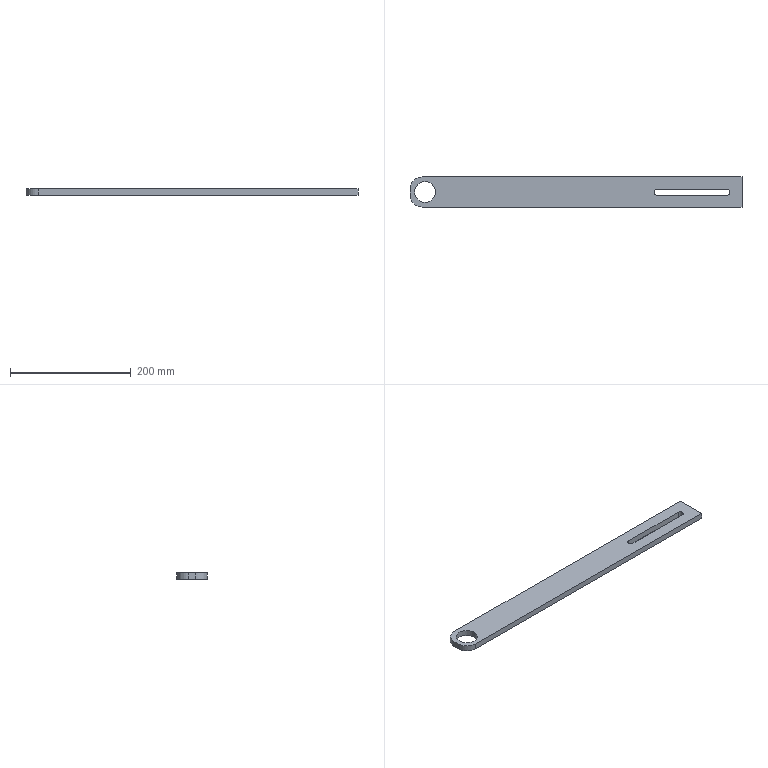Part | SolidWorks | features ICE 2, Extrusion 1, Fillet 1 | 1 solid | 18 faces | box 550 x 50 x 10 mm | volume 251336 mm3 | plane 10 | cylinder 8 | commonest cylinder face diameters 9 x4 35 x2 40 x2
STEP:
#1=CARTESIAN_POINT('',(-267.5,0.,0.));
#2=VERTEX_POINT('',#1);
#3=CARTESIAN_POINT('',(-232.5,0.,0.));
#4=VERTEX_POINT('',#3);
#5=CARTESIAN_POINT('',(-250.,0.,0.));
#6=DIRECTION('',(0.,0.,1.));
#7=DIRECTION('',(1.,0.,0.));
#8=AXIS2_PLACEMENT_3D('',#5,#6,#7);
#9=CIRCLE('',#8,17.5);
#10=EDGE_CURVE('',#2,#4,#9,.T.);
#11=ORIENTED_EDGE('',*,*,#10,.F.);
#12=CARTESIAN_POINT('',(-267.5,0.,10.));
#13=VERTEX_POINT('',#12);
#14=CARTESIAN_POINT('',(-267.5,0.,0.));
#15=DIRECTION('',(0.,0.,1.));
#16=VECTOR('',#15,1000.);
#17=LINE('',#14,#16);
#18=EDGE_CURVE('',#2,#13,#17,.T.);
#19=ORIENTED_EDGE('',*,*,#18,.T.);
#20=CARTESIAN_POINT('',(-232.5,0.,10.));
#21=VERTEX_POINT('',#20);
#22=CARTESIAN_POINT('',(-250.,0.,10.));
#23=DIRECTION('',(0.,0.,1.));
#24=DIRECTION('',(1.,0.,0.));
#25=AXIS2_PLACEMENT_3D('',#22,#23,#24);
#26=CIRCLE('',#25,17.5);
#27=EDGE_CURVE('',#13,#21,#26,.T.);
#28=ORIENTED_EDGE('',*,*,#27,.T.);
#29=CARTESIAN_POINT('',(-232.5,0.,0.));
#30=DIRECTION('',(0.,0.,1.));
#31=VECTOR('',#30,1000.);
#32=LINE('',#29,#31);
#33=EDGE_CURVE('',#4,#21,#32,.T.);
#34=ORIENTED_EDGE('',*,*,#33,.F.);
#35=EDGE_LOOP('',(#11,#19,#28,#34));
#36=FACE_OUTER_BOUND('',#35,.T.);
#37=CARTESIAN_POINT('',(-250.,0.,0.));
#38=DIRECTION('',(0.,0.,1.));
#39=DIRECTION('',(1.,0.,0.));
#40=AXIS2_PLACEMENT_3D('',#37,#38,#39);
#41=CYLINDRICAL_SURFACE('',#40,17.5);
#42=ADVANCED_FACE('',(#36),#41,.F.);
#43=CARTESIAN_POINT('',(-275.,5.,0.));
#44=VERTEX_POINT('',#43);
#45=CARTESIAN_POINT('',(-275.,-5.,0.));
#46=VERTEX_POINT('',#45);
#47=CARTESIAN_POINT('',(-275.,-25.,0.));
#48=DIRECTION('',(0.,-1.,0.));
#49=VECTOR('',#48,1000.);
#50=LINE('',#47,#49);
#51=EDGE_CURVE('',#44,#46,#50,.T.);
#52=ORIENTED_EDGE('',*,*,#51,.T.);
#53=CARTESIAN_POINT('',(-275.,-5.,10.));
#54=VERTEX_POINT('',#53);
#55=CARTESIAN_POINT('',(-275.,-5.,10.));
#56=DIRECTION('',(0.,0.,1.));
#57=VECTOR('',#56,1000.);
#58=LINE('',#55,#57);
#59=EDGE_CURVE('',#46,#54,#58,.T.);
#60=ORIENTED_EDGE('',*,*,#59,.T.);
#61=CARTESIAN_POINT('',(-275.,5.,10.));
#62=VERTEX_POINT('',#61);
#63=CARTESIAN_POINT('',(-275.,-25.,10.));
#64=DIRECTION('',(0.,-1.,0.));
#65=VECTOR('',#64,1000.);
#66=LINE('',#63,#65);
#67=EDGE_CURVE('',#62,#54,#66,.T.);
#68=ORIENTED_EDGE('',*,*,#67,.F.);
#69=CARTESIAN_POINT('',(-275.,5.,10.));
#70=DIRECTION('',(0.,0.,-1.));
#71=VECTOR('',#70,1000.);
#72=LINE('',#69,#71);
#73=EDGE_CURVE('',#62,#44,#72,.T.);
#74=ORIENTED_EDGE('',*,*,#73,.T.);
#75=EDGE_LOOP('',(#52,#60,#68,#74));
#76=FACE_OUTER_BOUND('',#75,.T.);
#77=CARTESIAN_POINT('',(-275.,-25.,10.));
#78=DIRECTION('',(1.,0.,0.));
#79=DIRECTION('',(0.,0.,-1.));
#80=AXIS2_PLACEMENT_3D('',#77,#78,#79);
#81=PLANE('',#80);
#82=ADVANCED_FACE('',(#76),#81,.F.);
#83=CARTESIAN_POINT('',(-255.,-25.,10.));
#84=VERTEX_POINT('',#83);
#85=CARTESIAN_POINT('',(275.,-25.,10.));
#86=VERTEX_POINT('',#85);
#87=CARTESIAN_POINT('',(275.,-25.,10.));
#88=DIRECTION('',(1.,0.,0.));
#89=VECTOR('',#88,1000.);
#90=LINE('',#87,#89);
#91=EDGE_CURVE('',#84,#86,#90,.T.);
#92=ORIENTED_EDGE('',*,*,#91,.F.);
#93=CARTESIAN_POINT('',(-255.,-25.,0.));
#94=VERTEX_POINT('',#93);
#95=CARTESIAN_POINT('',(-255.,-25.,10.));
#96=DIRECTION('',(0.,0.,-1.));
#97=VECTOR('',#96,1000.);
#98=LINE('',#95,#97);
#99=EDGE_CURVE('',#84,#94,#98,.T.);
#100=ORIENTED_EDGE('',*,*,#99,.T.);
#101=CARTESIAN_POINT('',(275.,-25.,0.));
#102=VERTEX_POINT('',#101);
#103=CARTESIAN_POINT('',(275.,-25.,0.));
#104=DIRECTION('',(1.,0.,0.));
#105=VECTOR('',#104,1000.);
#106=LINE('',#103,#105);
#107=EDGE_CURVE('',#94,#102,#106,.T.);
#108=ORIENTED_EDGE('',*,*,#107,.T.);
#109=CARTESIAN_POINT('',(275.,-25.,10.));
#110=DIRECTION('',(0.,0.,-1.));
#111=VECTOR('',#110,1000.);
#112=LINE('',#109,#111);
#113=EDGE_CURVE('',#86,#102,#112,.T.);
#114=ORIENTED_EDGE('',*,*,#113,.F.);
#115=EDGE_LOOP('',(#92,#100,#108,#114));
#116=FACE_OUTER_BOUND('',#115,.T.);
#117=CARTESIAN_POINT('',(275.,-25.,10.));
#118=DIRECTION('',(0.,1.,0.));
#119=DIRECTION('',(-1.,0.,0.));
#120=AXIS2_PLACEMENT_3D('',#117,#118,#119);
#121=PLANE('',#120);
#122=ADVANCED_FACE('',(#116),#121,.F.);
#123=CARTESIAN_POINT('',(275.,25.,0.));
#124=VERTEX_POINT('',#123);
#125=CARTESIAN_POINT('',(275.,-25.,0.));
#126=DIRECTION('',(0.,1.,0.));
#127=VECTOR('',#126,1000.);
#128=LINE('',#125,#127);
#129=EDGE_CURVE('',#102,#124,#128,.T.);
#130=ORIENTED_EDGE('',*,*,#129,.T.);
#131=CARTESIAN_POINT('',(275.,25.,10.));
#132=VERTEX_POINT('',#131);
#133=CARTESIAN_POINT('',(275.,25.,10.));
#134=DIRECTION('',(0.,0.,-1.));
#135=VECTOR('',#134,1000.);
#136=LINE('',#133,#135);
#137=EDGE_CURVE('',#132,#124,#136,.T.);
#138=ORIENTED_EDGE('',*,*,#137,.F.);
#139=CARTESIAN_POINT('',(275.,-25.,10.));
#140=DIRECTION('',(0.,1.,0.));
#141=VECTOR('',#140,1000.);
#142=LINE('',#139,#141);
#143=EDGE_CURVE('',#86,#132,#142,.T.);
#144=ORIENTED_EDGE('',*,*,#143,.F.);
#145=ORIENTED_EDGE('',*,*,#113,.T.);
#146=EDGE_LOOP('',(#130,#138,#144,#145));
#147=FACE_OUTER_BOUND('',#146,.T.);
#148=CARTESIAN_POINT('',(275.,-25.,10.));
#149=DIRECTION('',(-1.,0.,0.));
#150=DIRECTION('',(0.,0.,1.));
#151=AXIS2_PLACEMENT_3D('',#148,#149,#150);
#152=PLANE('',#151);
#153=ADVANCED_FACE('',(#147),#152,.F.);
#154=CARTESIAN_POINT('',(-255.,25.,0.));
#155=VERTEX_POINT('',#154);
#156=CARTESIAN_POINT('',(275.,25.,0.));
#157=DIRECTION('',(-1.,0.,0.));
#158=VECTOR('',#157,1000.);
#159=LINE('',#156,#158);
#160=EDGE_CURVE('',#124,#155,#159,.T.);
#161=ORIENTED_EDGE('',*,*,#160,.T.);
#162=CARTESIAN_POINT('',(-255.,25.,10.));
#163=VERTEX_POINT('',#162);
#164=CARTESIAN_POINT('',(-255.,25.,10.));
#165=DIRECTION('',(0.,0.,1.));
#166=VECTOR('',#165,1000.);
#167=LINE('',#164,#166);
#168=EDGE_CURVE('',#155,#163,#167,.T.);
#169=ORIENTED_EDGE('',*,*,#168,.T.);
#170=CARTESIAN_POINT('',(275.,25.,10.));
#171=DIRECTION('',(-1.,0.,0.));
#172=VECTOR('',#171,1000.);
#173=LINE('',#170,#172);
#174=EDGE_CURVE('',#132,#163,#173,.T.);
#175=ORIENTED_EDGE('',*,*,#174,.F.);
#176=ORIENTED_EDGE('',*,*,#137,.T.);
#177=EDGE_LOOP('',(#161,#169,#175,#176));
#178=FACE_OUTER_BOUND('',#177,.T.);
#179=CARTESIAN_POINT('',(275.,25.,10.));
#180=DIRECTION('',(0.,-1.,0.));
#181=DIRECTION('',(1.,0.,0.));
#182=AXIS2_PLACEMENT_3D('',#179,#180,#181);
#183=PLANE('',#182);
#184=ADVANCED_FACE('',(#178),#183,.F.);
#185=CARTESIAN_POINT('',(250.1,-5.341,10.));
#186=VERTEX_POINT('',#185);
#187=CARTESIAN_POINT('',(254.6,-0.841,10.));
#188=VERTEX_POINT('',#187);
#189=CARTESIAN_POINT('',(250.1,-0.841,10.));
#190=DIRECTION('',(0.,0.,1.));
#191=DIRECTION('',(1.,0.,0.));
#192=AXIS2_PLACEMENT_3D('',#189,#190,#191);
#193=CIRCLE('',#192,4.5);
#194=EDGE_CURVE('',#186,#188,#193,.T.);
#195=ORIENTED_EDGE('',*,*,#194,.F.);
#196=CARTESIAN_POINT('',(134.1,-5.341,10.));
#197=VERTEX_POINT('',#196);
#198=CARTESIAN_POINT('',(250.1,-5.341,10.));
#199=DIRECTION('',(1.,0.,0.));
#200=VECTOR('',#199,1000.);
#201=LINE('',#198,#200);
#202=EDGE_CURVE('',#197,#186,#201,.T.);
#203=ORIENTED_EDGE('',*,*,#202,.F.);
#204=CARTESIAN_POINT('',(129.6,-0.841,10.));
#205=VERTEX_POINT('',#204);
#206=CARTESIAN_POINT('',(134.1,-0.841,10.));
#207=DIRECTION('',(0.,0.,1.));
#208=DIRECTION('',(-1.,0.,0.));
#209=AXIS2_PLACEMENT_3D('',#206,#207,#208);
#210=CIRCLE('',#209,4.5);
#211=EDGE_CURVE('',#205,#197,#210,.T.);
#212=ORIENTED_EDGE('',*,*,#211,.F.);
#213=CARTESIAN_POINT('',(129.6,0.159,10.));
#214=VERTEX_POINT('',#213);
#215=CARTESIAN_POINT('',(129.6,-0.841,10.));
#216=DIRECTION('',(0.,-1.,0.));
#217=VECTOR('',#216,1000.);
#218=LINE('',#215,#217);
#219=EDGE_CURVE('',#214,#205,#218,.T.);
#220=ORIENTED_EDGE('',*,*,#219,.F.);
#221=CARTESIAN_POINT('',(134.1,4.659,10.));
#222=VERTEX_POINT('',#221);
#223=CARTESIAN_POINT('',(134.1,0.159,10.));
#224=DIRECTION('',(0.,0.,1.));
#225=DIRECTION('',(1.,0.,0.));
#226=AXIS2_PLACEMENT_3D('',#223,#224,#225);
#227=CIRCLE('',#226,4.5);
#228=EDGE_CURVE('',#222,#214,#227,.T.);
#229=ORIENTED_EDGE('',*,*,#228,.F.);
#230=CARTESIAN_POINT('',(250.1,4.659,10.));
#231=VERTEX_POINT('',#230);
#232=CARTESIAN_POINT('',(250.1,4.659,10.));
#233=DIRECTION('',(-1.,0.,0.));
#234=VECTOR('',#233,1000.);
#235=LINE('',#232,#234);
#236=EDGE_CURVE('',#231,#222,#235,.T.);
#237=ORIENTED_EDGE('',*,*,#236,.F.);
#238=CARTESIAN_POINT('',(254.6,0.159,10.));
#239=VERTEX_POINT('',#238);
#240=CARTESIAN_POINT('',(250.1,0.159,10.));
#241=DIRECTION('',(0.,0.,1.));
#242=DIRECTION('',(1.,0.,0.));
#243=AXIS2_PLACEMENT_3D('',#240,#241,#242);
#244=CIRCLE('',#243,4.5);
#245=EDGE_CURVE('',#239,#231,#244,.T.);
#246=ORIENTED_EDGE('',*,*,#245,.F.);
#247=CARTESIAN_POINT('',(254.6,-0.841,10.));
#248=DIRECTION('',(0.,1.,0.));
#249=VECTOR('',#248,1000.);
#250=LINE('',#247,#249);
#251=EDGE_CURVE('',#188,#239,#250,.T.);
#252=ORIENTED_EDGE('',*,*,#251,.F.);
#253=EDGE_LOOP('',(#195,#203,#212,#220,#229,#237,#246,#252));
#254=FACE_BOUND('',#253,.T.);
#255=CARTESIAN_POINT('',(-250.,0.,10.));
#256=DIRECTION('',(0.,0.,1.));
#257=DIRECTION('',(1.,0.,0.));
#258=AXIS2_PLACEMENT_3D('',#255,#256,#257);
#259=CIRCLE('',#258,17.5);
#260=EDGE_CURVE('',#21,#13,#259,.T.);
#261=ORIENTED_EDGE('',*,*,#260,.F.);
#262=ORIENTED_EDGE('',*,*,#27,.F.);
#263=EDGE_LOOP('',(#261,#262));
#264=FACE_BOUND('',#263,.T.);
#265=ORIENTED_EDGE('',*,*,#67,.T.);
#266=CARTESIAN_POINT('',(-255.,-5.,10.));
#267=DIRECTION('',(0.,0.,1.));
#268=DIRECTION('',(1.,0.,0.));
#269=AXIS2_PLACEMENT_3D('',#266,#267,#268);
#270=CIRCLE('',#269,20.);
#271=EDGE_CURVE('',#54,#84,#270,.T.);
#272=ORIENTED_EDGE('',*,*,#271,.T.);
#273=ORIENTED_EDGE('',*,*,#91,.T.);
#274=ORIENTED_EDGE('',*,*,#143,.T.);
#275=ORIENTED_EDGE('',*,*,#174,.T.);
#276=CARTESIAN_POINT('',(-255.,5.,10.));
#277=DIRECTION('',(0.,0.,1.));
#278=DIRECTION('',(1.,0.,0.));
#279=AXIS2_PLACEMENT_3D('',#276,#277,#278);
#280=CIRCLE('',#279,20.);
#281=EDGE_CURVE('',#163,#62,#280,.T.);
#282=ORIENTED_EDGE('',*,*,#281,.T.);
#283=EDGE_LOOP('',(#265,#272,#273,#274,#275,#282));
#284=FACE_OUTER_BOUND('',#283,.T.);
#285=CARTESIAN_POINT('',(-275.,25.,10.));
#286=DIRECTION('',(0.,0.,1.));
#287=DIRECTION('',(1.,0.,0.));
#288=AXIS2_PLACEMENT_3D('',#285,#286,#287);
#289=PLANE('',#288);
#290=ADVANCED_FACE('',(#254,#264,#284),#289,.T.);
#291=CARTESIAN_POINT('',(134.1,-5.341,0.));
#292=VERTEX_POINT('',#291);
#293=CARTESIAN_POINT('',(250.1,-5.341,0.));
#294=VERTEX_POINT('',#293);
#295=CARTESIAN_POINT('',(250.1,-5.341,0.));
#296=DIRECTION('',(1.,0.,0.));
#297=VECTOR('',#296,1000.);
#298=LINE('',#295,#297);
#299=EDGE_CURVE('',#292,#294,#298,.T.);
#300=ORIENTED_EDGE('',*,*,#299,.T.);
#301=CARTESIAN_POINT('',(254.6,-0.841,0.));
#302=VERTEX_POINT('',#301);
#303=CARTESIAN_POINT('',(250.1,-0.841,0.));
#304=DIRECTION('',(0.,0.,1.));
#305=DIRECTION('',(1.,0.,0.));
#306=AXIS2_PLACEMENT_3D('',#303,#304,#305);
#307=CIRCLE('',#306,4.5);
#308=EDGE_CURVE('',#294,#302,#307,.T.);
#309=ORIENTED_EDGE('',*,*,#308,.T.);
#310=CARTESIAN_POINT('',(254.6,0.159,0.));
#311=VERTEX_POINT('',#310);
#312=CARTESIAN_POINT('',(254.6,-0.841,0.));
#313=DIRECTION('',(0.,1.,0.));
#314=VECTOR('',#313,1000.);
#315=LINE('',#312,#314);
#316=EDGE_CURVE('',#302,#311,#315,.T.);
#317=ORIENTED_EDGE('',*,*,#316,.T.);
#318=CARTESIAN_POINT('',(250.1,4.659,0.));
#319=VERTEX_POINT('',#318);
#320=CARTESIAN_POINT('',(250.1,0.159,0.));
#321=DIRECTION('',(0.,0.,1.));
#322=DIRECTION('',(1.,0.,0.));
#323=AXIS2_PLACEMENT_3D('',#320,#321,#322);
#324=CIRCLE('',#323,4.5);
#325=EDGE_CURVE('',#311,#319,#324,.T.);
#326=ORIENTED_EDGE('',*,*,#325,.T.);
#327=CARTESIAN_POINT('',(134.1,4.659,0.));
#328=VERTEX_POINT('',#327);
#329=CARTESIAN_POINT('',(250.1,4.659,0.));
#330=DIRECTION('',(-1.,0.,0.));
#331=VECTOR('',#330,1000.);
#332=LINE('',#329,#331);
#333=EDGE_CURVE('',#319,#328,#332,.T.);
#334=ORIENTED_EDGE('',*,*,#333,.T.);
#335=CARTESIAN_POINT('',(129.6,0.159,0.));
#336=VERTEX_POINT('',#335);
#337=CARTESIAN_POINT('',(134.1,0.159,0.));
#338=DIRECTION('',(0.,0.,1.));
#339=DIRECTION('',(1.,0.,0.));
#340=AXIS2_PLACEMENT_3D('',#337,#338,#339);
#341=CIRCLE('',#340,4.5);
#342=EDGE_CURVE('',#328,#336,#341,.T.);
#343=ORIENTED_EDGE('',*,*,#342,.T.);
#344=CARTESIAN_POINT('',(129.6,-0.841,0.));
#345=VERTEX_POINT('',#344);
#346=CARTESIAN_POINT('',(129.6,-0.841,0.));
#347=DIRECTION('',(0.,-1.,0.));
#348=VECTOR('',#347,1000.);
#349=LINE('',#346,#348);
#350=EDGE_CURVE('',#336,#345,#349,.T.);
#351=ORIENTED_EDGE('',*,*,#350,.T.);
#352=CARTESIAN_POINT('',(134.1,-0.841,0.));
#353=DIRECTION('',(0.,0.,1.));
#354=DIRECTION('',(-1.,0.,0.));
#355=AXIS2_PLACEMENT_3D('',#352,#353,#354);
#356=CIRCLE('',#355,4.5);
#357=EDGE_CURVE('',#345,#292,#356,.T.);
#358=ORIENTED_EDGE('',*,*,#357,.T.);
#359=EDGE_LOOP('',(#300,#309,#317,#326,#334,#343,#351,#358));
#360=FACE_BOUND('',#359,.T.);
#361=CARTESIAN_POINT('',(-250.,0.,0.));
#362=DIRECTION('',(0.,0.,1.));
#363=DIRECTION('',(1.,0.,0.));
#364=AXIS2_PLACEMENT_3D('',#361,#362,#363);
#365=CIRCLE('',#364,17.5);
#366=EDGE_CURVE('',#4,#2,#365,.T.);
#367=ORIENTED_EDGE('',*,*,#366,.T.);
#368=ORIENTED_EDGE('',*,*,#10,.T.);
#369=EDGE_LOOP('',(#367,#368));
#370=FACE_BOUND('',#369,.T.);
#371=ORIENTED_EDGE('',*,*,#107,.F.);
#372=CARTESIAN_POINT('',(-255.,-5.,0.));
#373=DIRECTION('',(0.,0.,-1.));
#374=DIRECTION('',(1.,0.,0.));
#375=AXIS2_PLACEMENT_3D('',#372,#373,#374);
#376=CIRCLE('',#375,20.);
#377=EDGE_CURVE('',#94,#46,#376,.T.);
#378=ORIENTED_EDGE('',*,*,#377,.T.);
#379=ORIENTED_EDGE('',*,*,#51,.F.);
#380=CARTESIAN_POINT('',(-255.,5.,0.));
#381=DIRECTION('',(0.,0.,-1.));
#382=DIRECTION('',(1.,0.,0.));
#383=AXIS2_PLACEMENT_3D('',#380,#381,#382);
#384=CIRCLE('',#383,20.);
#385=EDGE_CURVE('',#44,#155,#384,.T.);
#386=ORIENTED_EDGE('',*,*,#385,.T.);
#387=ORIENTED_EDGE('',*,*,#160,.F.);
#388=ORIENTED_EDGE('',*,*,#129,.F.);
#389=EDGE_LOOP('',(#371,#378,#379,#386,#387,#388));
#390=FACE_OUTER_BOUND('',#389,.T.);
#391=CARTESIAN_POINT('',(-275.,25.,0.));
#392=DIRECTION('',(0.,0.,1.));
#393=DIRECTION('',(1.,0.,0.));
#394=AXIS2_PLACEMENT_3D('',#391,#392,#393);
#395=PLANE('',#394);
#396=ADVANCED_FACE('',(#360,#370,#390),#395,.F.);
#397=ORIENTED_EDGE('',*,*,#18,.F.);
#398=ORIENTED_EDGE('',*,*,#366,.F.);
#399=ORIENTED_EDGE('',*,*,#33,.T.);
#400=ORIENTED_EDGE('',*,*,#260,.T.);
#401=EDGE_LOOP('',(#397,#398,#399,#400));
#402=FACE_OUTER_BOUND('',#401,.T.);
#403=CARTESIAN_POINT('',(-250.,0.,0.));
#404=DIRECTION('',(0.,0.,1.));
#405=DIRECTION('',(1.,0.,0.));
#406=AXIS2_PLACEMENT_3D('',#403,#404,#405);
#407=CYLINDRICAL_SURFACE('',#406,17.5);
#408=ADVANCED_FACE('',(#402),#407,.F.);
#409=ORIENTED_EDGE('',*,*,#194,.T.);
#410=CARTESIAN_POINT('',(254.6,-0.841,0.));
#411=DIRECTION('',(0.,0.,1.));
#412=VECTOR('',#411,1000.);
#413=LINE('',#410,#412);
#414=EDGE_CURVE('',#302,#188,#413,.T.);
#415=ORIENTED_EDGE('',*,*,#414,.F.);
#416=ORIENTED_EDGE('',*,*,#308,.F.);
#417=CARTESIAN_POINT('',(250.1,-5.341,0.));
#418=DIRECTION('',(0.,0.,1.));
#419=VECTOR('',#418,1000.);
#420=LINE('',#417,#419);
#421=EDGE_CURVE('',#294,#186,#420,.T.);
#422=ORIENTED_EDGE('',*,*,#421,.T.);
#423=EDGE_LOOP('',(#409,#415,#416,#422));
#424=FACE_OUTER_BOUND('',#423,.T.);
#425=CARTESIAN_POINT('',(250.1,-0.841,0.));
#426=DIRECTION('',(0.,0.,1.));
#427=DIRECTION('',(1.,0.,0.));
#428=AXIS2_PLACEMENT_3D('',#425,#426,#427);
#429=CYLINDRICAL_SURFACE('',#428,4.5);
#430=ADVANCED_FACE('',(#424),#429,.F.);
#431=ORIENTED_EDGE('',*,*,#202,.T.);
#432=ORIENTED_EDGE('',*,*,#421,.F.);
#433=ORIENTED_EDGE('',*,*,#299,.F.);
#434=CARTESIAN_POINT('',(134.1,-5.341,0.));
#435=DIRECTION('',(0.,0.,1.));
#436=VECTOR('',#435,1000.);
#437=LINE('',#434,#436);
#438=EDGE_CURVE('',#292,#197,#437,.T.);
#439=ORIENTED_EDGE('',*,*,#438,.T.);
#440=EDGE_LOOP('',(#431,#432,#433,#439));
#441=FACE_OUTER_BOUND('',#440,.T.);
#442=CARTESIAN_POINT('',(250.1,-5.341,0.));
#443=DIRECTION('',(0.,-1.,0.));
#444=DIRECTION('',(1.,0.,0.));
#445=AXIS2_PLACEMENT_3D('',#442,#443,#444);
#446=PLANE('',#445);
#447=ADVANCED_FACE('',(#441),#446,.F.);
#448=ORIENTED_EDGE('',*,*,#211,.T.);
#449=ORIENTED_EDGE('',*,*,#438,.F.);
#450=ORIENTED_EDGE('',*,*,#357,.F.);
#451=CARTESIAN_POINT('',(129.6,-0.841,0.));
#452=DIRECTION('',(0.,0.,1.));
#453=VECTOR('',#452,1000.);
#454=LINE('',#451,#453);
#455=EDGE_CURVE('',#345,#205,#454,.T.);
#456=ORIENTED_EDGE('',*,*,#455,.T.);
#457=EDGE_LOOP('',(#448,#449,#450,#456));
#458=FACE_OUTER_BOUND('',#457,.T.);
#459=CARTESIAN_POINT('',(134.1,-0.841,0.));
#460=DIRECTION('',(0.,0.,1.));
#461=DIRECTION('',(1.,0.,0.));
#462=AXIS2_PLACEMENT_3D('',#459,#460,#461);
#463=CYLINDRICAL_SURFACE('',#462,4.5);
#464=ADVANCED_FACE('',(#458),#463,.F.);
#465=ORIENTED_EDGE('',*,*,#219,.T.);
#466=ORIENTED_EDGE('',*,*,#455,.F.);
#467=ORIENTED_EDGE('',*,*,#350,.F.);
#468=CARTESIAN_POINT('',(129.6,0.159,0.));
#469=DIRECTION('',(0.,0.,1.));
#470=VECTOR('',#469,1000.);
#471=LINE('',#468,#470);
#472=EDGE_CURVE('',#336,#214,#471,.T.);
#473=ORIENTED_EDGE('',*,*,#472,.T.);
#474=EDGE_LOOP('',(#465,#466,#467,#473));
#475=FACE_OUTER_BOUND('',#474,.T.);
#476=CARTESIAN_POINT('',(129.6,-0.841,0.));
#477=DIRECTION('',(-1.,0.,0.));
#478=DIRECTION('',(0.,0.,1.));
#479=AXIS2_PLACEMENT_3D('',#476,#477,#478);
#480=PLANE('',#479);
#481=ADVANCED_FACE('',(#475),#480,.F.);
#482=ORIENTED_EDGE('',*,*,#228,.T.);
#483=ORIENTED_EDGE('',*,*,#472,.F.);
#484=ORIENTED_EDGE('',*,*,#342,.F.);
#485=CARTESIAN_POINT('',(134.1,4.659,0.));
#486=DIRECTION('',(0.,0.,1.));
#487=VECTOR('',#486,1000.);
#488=LINE('',#485,#487);
#489=EDGE_CURVE('',#328,#222,#488,.T.);
#490=ORIENTED_EDGE('',*,*,#489,.T.);
#491=EDGE_LOOP('',(#482,#483,#484,#490));
#492=FACE_OUTER_BOUND('',#491,.T.);
#493=CARTESIAN_POINT('',(134.1,0.159,0.));
#494=DIRECTION('',(0.,0.,1.));
#495=DIRECTION('',(1.,0.,0.));
#496=AXIS2_PLACEMENT_3D('',#493,#494,#495);
#497=CYLINDRICAL_SURFACE('',#496,4.5);
#498=ADVANCED_FACE('',(#492),#497,.F.);
#499=ORIENTED_EDGE('',*,*,#236,.T.);
#500=ORIENTED_EDGE('',*,*,#489,.F.);
#501=ORIENTED_EDGE('',*,*,#333,.F.);
#502=CARTESIAN_POINT('',(250.1,4.659,0.));
#503=DIRECTION('',(0.,0.,1.));
#504=VECTOR('',#503,1000.);
#505=LINE('',#502,#504);
#506=EDGE_CURVE('',#319,#231,#505,.T.);
#507=ORIENTED_EDGE('',*,*,#506,.T.);
#508=EDGE_LOOP('',(#499,#500,#501,#507));
#509=FACE_OUTER_BOUND('',#508,.T.);
#510=CARTESIAN_POINT('',(250.1,4.659,0.));
#511=DIRECTION('',(0.,1.,0.));
#512=DIRECTION('',(-1.,0.,0.));
#513=AXIS2_PLACEMENT_3D('',#510,#511,#512);
#514=PLANE('',#513);
#515=ADVANCED_FACE('',(#509),#514,.F.);
#516=ORIENTED_EDGE('',*,*,#245,.T.);
#517=ORIENTED_EDGE('',*,*,#506,.F.);
#518=ORIENTED_EDGE('',*,*,#325,.F.);
#519=CARTESIAN_POINT('',(254.6,0.159,0.));
#520=DIRECTION('',(0.,0.,1.));
#521=VECTOR('',#520,1000.);
#522=LINE('',#519,#521);
#523=EDGE_CURVE('',#311,#239,#522,.T.);
#524=ORIENTED_EDGE('',*,*,#523,.T.);
#525=EDGE_LOOP('',(#516,#517,#518,#524));
#526=FACE_OUTER_BOUND('',#525,.T.);
#527=CARTESIAN_POINT('',(250.1,0.159,0.));
#528=DIRECTION('',(0.,0.,1.));
#529=DIRECTION('',(1.,0.,0.));
#530=AXIS2_PLACEMENT_3D('',#527,#528,#529);
#531=CYLINDRICAL_SURFACE('',#530,4.5);
#532=ADVANCED_FACE('',(#526),#531,.F.);
#533=ORIENTED_EDGE('',*,*,#251,.T.);
#534=ORIENTED_EDGE('',*,*,#523,.F.);
#535=ORIENTED_EDGE('',*,*,#316,.F.);
#536=ORIENTED_EDGE('',*,*,#414,.T.);
#537=EDGE_LOOP('',(#533,#534,#535,#536));
#538=FACE_OUTER_BOUND('',#537,.T.);
#539=CARTESIAN_POINT('',(254.6,-0.841,0.));
#540=DIRECTION('',(1.,0.,0.));
#541=DIRECTION('',(0.,0.,-1.));
#542=AXIS2_PLACEMENT_3D('',#539,#540,#541);
#543=PLANE('',#542);
#544=ADVANCED_FACE('',(#538),#543,.F.);
#545=ORIENTED_EDGE('',*,*,#271,.F.);
#546=ORIENTED_EDGE('',*,*,#59,.F.);
#547=ORIENTED_EDGE('',*,*,#377,.F.);
#548=ORIENTED_EDGE('',*,*,#99,.F.);
#549=EDGE_LOOP('',(#545,#546,#547,#548));
#550=FACE_OUTER_BOUND('',#549,.T.);
#551=CARTESIAN_POINT('',(-255.,-5.,10.));
#552=DIRECTION('',(0.,0.,-1.));
#553=DIRECTION('',(-1.,0.,0.));
#554=AXIS2_PLACEMENT_3D('',#551,#552,#553);
#555=CYLINDRICAL_SURFACE('',#554,20.);
#556=ADVANCED_FACE('',(#550),#555,.T.);
#557=ORIENTED_EDGE('',*,*,#281,.F.);
#558=ORIENTED_EDGE('',*,*,#168,.F.);
#559=ORIENTED_EDGE('',*,*,#385,.F.);
#560=ORIENTED_EDGE('',*,*,#73,.F.);
#561=EDGE_LOOP('',(#557,#558,#559,#560));
#562=FACE_OUTER_BOUND('',#561,.T.);
#563=CARTESIAN_POINT('',(-255.,5.,10.));
#564=DIRECTION('',(0.,0.,-1.));
#565=DIRECTION('',(-1.,0.,0.));
#566=AXIS2_PLACEMENT_3D('',#563,#564,#565);
#567=CYLINDRICAL_SURFACE('',#566,20.);
#568=ADVANCED_FACE('',(#562),#567,.T.);
#569=CLOSED_SHELL('',(#42,#82,#122,#153,#184,#290,#396,#408,#430,#447,#464,#481,#498,#515,#532,#544,#556,#568));
#570=MANIFOLD_SOLID_BREP('',#569);
#571=CARTESIAN_POINT('',(0.,0.,0.));
#572=DIRECTION('',(0.,0.,1.));
#573=DIRECTION('',(1.,0.,0.));
#574=AXIS2_PLACEMENT_3D('',#571,#572,#573);
#575=(LENGTH_UNIT()NAMED_UNIT(*)SI_UNIT(.MILLI.,.METRE.));
#576=UNCERTAINTY_MEASURE_WITH_UNIT(LENGTH_MEASURE(0.00001),#575,'','');
#577=(NAMED_UNIT(*)PLANE_ANGLE_UNIT()SI_UNIT($,.RADIAN.));
#578=(NAMED_UNIT(*)SI_UNIT($,.STERADIAN.)SOLID_ANGLE_UNIT());
#579=(GEOMETRIC_REPRESENTATION_CONTEXT(3)GLOBAL_UNCERTAINTY_ASSIGNED_CONTEXT((#576))GLOBAL_UNIT_ASSIGNED_CONTEXT((#575,#577,#578))REPRESENTATION_CONTEXT('',''));
#580=ADVANCED_BREP_SHAPE_REPRESENTATION('',(#570,#574),#579);